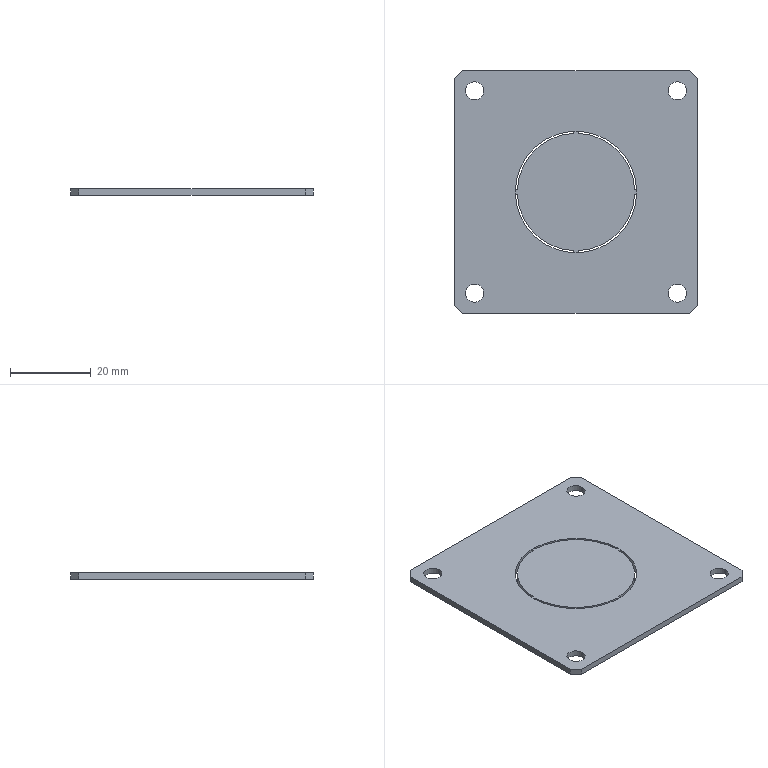Part | STEP file | Ethernet port | 2 solids | 38 faces | box 60 x 60 x 1.5 mm | volume 5226 mm3 | plane 24 | cylinder 14 | commonest cylinder face diameters 4.5 x8 29 x4 30 x2